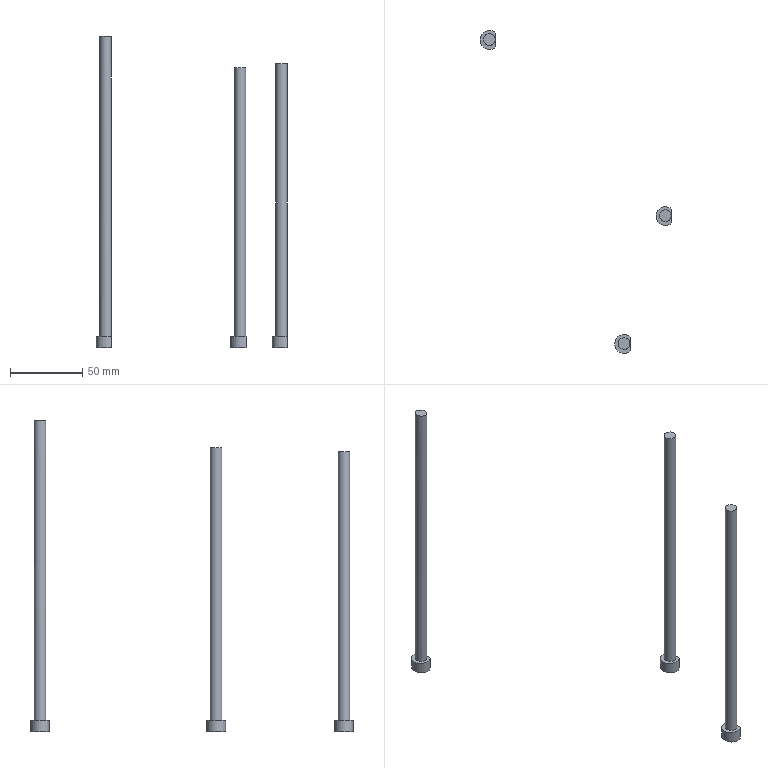Part | STEP file | DDZ8 | 3 solids | 18 faces | box 132.5 x 223 x 215.546 mm | volume 32090 mm3 | plane 11 | cylinder 7 | commonest cylinder face diameters 8 x3 13 x3 6922 x1